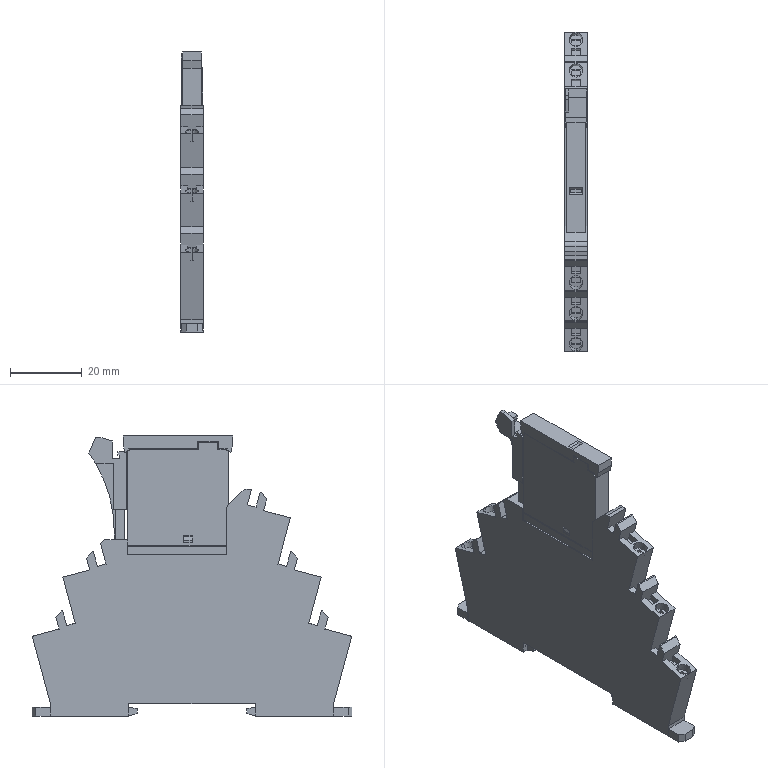Part | STEP file | 4 solids | 387 faces | box 6.2 x 88.87 x 77.9 mm | volume 26675 mm3 | plane 371 | cylinder 16 | commonest cylinder face diameters 3.9 x10 0.2 x1 0.8 x1 1 x1 2 x1 4 x1